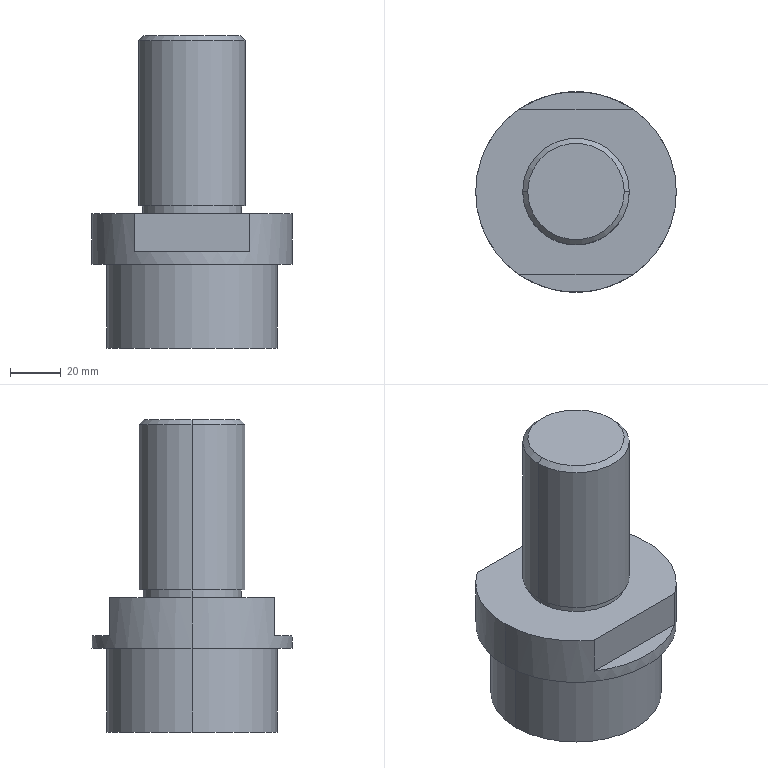Part | SolidWorks | features ICE 4, Chamfer 1, Extrusion 1 | 1 solid | 19 faces | box 79 x 79 x 123 mm | volume 304126 mm3 | plane 9 | cylinder 8 | cone 2 | commonest cylinder face diameters 39 x2 42 x2 67 x2 79 x2
STEP:
#1=CARTESIAN_POINT('',(19.,0.,123.));
#2=VERTEX_POINT('',#1);
#3=CARTESIAN_POINT('',(-19.,0.,123.));
#4=VERTEX_POINT('',#3);
#5=CARTESIAN_POINT('',(0.,0.,123.));
#6=DIRECTION('',(0.,0.,1.));
#7=DIRECTION('',(1.,0.,0.));
#8=AXIS2_PLACEMENT_3D('',#5,#6,#7);
#9=CIRCLE('',#8,19.);
#10=EDGE_CURVE('',#2,#4,#9,.T.);
#11=ORIENTED_EDGE('',*,*,#10,.F.);
#12=CARTESIAN_POINT('',(21.,0.,121.));
#13=VERTEX_POINT('',#12);
#14=CARTESIAN_POINT('',(19.,0.,123.));
#15=DIRECTION('',(0.7071,0.,-0.7071));
#16=VECTOR('',#15,1000.);
#17=LINE('',#14,#16);
#18=EDGE_CURVE('',#2,#13,#17,.T.);
#19=ORIENTED_EDGE('',*,*,#18,.T.);
#20=CARTESIAN_POINT('',(-21.,0.,121.));
#21=VERTEX_POINT('',#20);
#22=CARTESIAN_POINT('',(0.,0.,121.));
#23=DIRECTION('',(0.,0.,-1.));
#24=DIRECTION('',(1.,0.,0.));
#25=AXIS2_PLACEMENT_3D('',#22,#23,#24);
#26=CIRCLE('',#25,21.);
#27=EDGE_CURVE('',#21,#13,#26,.T.);
#28=ORIENTED_EDGE('',*,*,#27,.F.);
#29=CARTESIAN_POINT('',(-19.,0.,123.));
#30=DIRECTION('',(-0.7071,0.,-0.7071));
#31=VECTOR('',#30,1000.);
#32=LINE('',#29,#31);
#33=EDGE_CURVE('',#4,#21,#32,.T.);
#34=ORIENTED_EDGE('',*,*,#33,.F.);
#35=EDGE_LOOP('',(#11,#19,#28,#34));
#36=FACE_OUTER_BOUND('',#35,.T.);
#37=CARTESIAN_POINT('',(0.,0.,123.));
#38=DIRECTION('',(0.,0.,-1.));
#39=DIRECTION('',(-1.,0.,0.));
#40=AXIS2_PLACEMENT_3D('',#37,#38,#39);
#41=CONICAL_SURFACE('',#40,19.,0.7854);
#42=ADVANCED_FACE('',(#36),#41,.T.);
#43=ORIENTED_EDGE('',*,*,#27,.T.);
#44=CARTESIAN_POINT('',(21.,0.,56.));
#45=VERTEX_POINT('',#44);
#46=CARTESIAN_POINT('',(21.,0.,123.));
#47=DIRECTION('',(0.,0.,-1.));
#48=VECTOR('',#47,1000.);
#49=LINE('',#46,#48);
#50=EDGE_CURVE('',#13,#45,#49,.T.);
#51=ORIENTED_EDGE('',*,*,#50,.T.);
#52=CARTESIAN_POINT('',(-21.,0.,56.));
#53=VERTEX_POINT('',#52);
#54=CARTESIAN_POINT('',(0.,0.,56.));
#55=DIRECTION('',(0.,0.,1.));
#56=DIRECTION('',(1.,0.,0.));
#57=AXIS2_PLACEMENT_3D('',#54,#55,#56);
#58=CIRCLE('',#57,21.);
#59=EDGE_CURVE('',#45,#53,#58,.T.);
#60=ORIENTED_EDGE('',*,*,#59,.T.);
#61=CARTESIAN_POINT('',(-21.,0.,123.));
#62=DIRECTION('',(0.,0.,-1.));
#63=VECTOR('',#62,1000.);
#64=LINE('',#61,#63);
#65=EDGE_CURVE('',#21,#53,#64,.T.);
#66=ORIENTED_EDGE('',*,*,#65,.F.);
#67=EDGE_LOOP('',(#43,#51,#60,#66));
#68=FACE_OUTER_BOUND('',#67,.T.);
#69=CARTESIAN_POINT('',(0.,0.,123.));
#70=DIRECTION('',(0.,0.,-1.));
#71=DIRECTION('',(-1.,0.,0.));
#72=AXIS2_PLACEMENT_3D('',#69,#70,#71);
#73=CYLINDRICAL_SURFACE('',#72,21.);
#74=ADVANCED_FACE('',(#68),#73,.T.);
#75=CARTESIAN_POINT('',(19.5,0.,56.));
#76=VERTEX_POINT('',#75);
#77=CARTESIAN_POINT('',(-19.5,0.,56.));
#78=VERTEX_POINT('',#77);
#79=CARTESIAN_POINT('',(0.,0.,56.));
#80=DIRECTION('',(0.,0.,1.));
#81=DIRECTION('',(1.,0.,0.));
#82=AXIS2_PLACEMENT_3D('',#79,#80,#81);
#83=CIRCLE('',#82,19.5);
#84=EDGE_CURVE('',#76,#78,#83,.T.);
#85=ORIENTED_EDGE('',*,*,#84,.F.);
#86=CARTESIAN_POINT('',(19.5,0.,53.));
#87=VERTEX_POINT('',#86);
#88=CARTESIAN_POINT('',(19.5,0.,56.));
#89=DIRECTION('',(0.,0.,-1.));
#90=VECTOR('',#89,1000.);
#91=LINE('',#88,#90);
#92=EDGE_CURVE('',#76,#87,#91,.T.);
#93=ORIENTED_EDGE('',*,*,#92,.T.);
#94=CARTESIAN_POINT('',(-19.5,0.,53.));
#95=VERTEX_POINT('',#94);
#96=CARTESIAN_POINT('',(0.,0.,53.));
#97=DIRECTION('',(0.,0.,1.));
#98=DIRECTION('',(1.,0.,0.));
#99=AXIS2_PLACEMENT_3D('',#96,#97,#98);
#100=CIRCLE('',#99,19.5);
#101=EDGE_CURVE('',#87,#95,#100,.T.);
#102=ORIENTED_EDGE('',*,*,#101,.T.);
#103=CARTESIAN_POINT('',(-19.5,0.,56.));
#104=DIRECTION('',(0.,0.,-1.));
#105=VECTOR('',#104,1000.);
#106=LINE('',#103,#105);
#107=EDGE_CURVE('',#78,#95,#106,.T.);
#108=ORIENTED_EDGE('',*,*,#107,.F.);
#109=EDGE_LOOP('',(#85,#93,#102,#108));
#110=FACE_OUTER_BOUND('',#109,.T.);
#111=CARTESIAN_POINT('',(0.,0.,56.));
#112=DIRECTION('',(0.,0.,-1.));
#113=DIRECTION('',(-1.,0.,0.));
#114=AXIS2_PLACEMENT_3D('',#111,#112,#113);
#115=CYLINDRICAL_SURFACE('',#114,19.5);
#116=ADVANCED_FACE('',(#110),#115,.T.);
#117=CARTESIAN_POINT('',(39.5,0.,53.));
#118=VERTEX_POINT('',#117);
#119=CARTESIAN_POINT('',(22.45,32.5,53.));
#120=VERTEX_POINT('',#119);
#121=CARTESIAN_POINT('',(0.,0.,53.));
#122=DIRECTION('',(0.,0.,1.));
#123=DIRECTION('',(1.,0.,0.));
#124=AXIS2_PLACEMENT_3D('',#121,#122,#123);
#125=CIRCLE('',#124,39.5);
#126=EDGE_CURVE('',#118,#120,#125,.T.);
#127=ORIENTED_EDGE('',*,*,#126,.F.);
#128=CARTESIAN_POINT('',(39.5,0.,33.));
#129=VERTEX_POINT('',#128);
#130=CARTESIAN_POINT('',(39.5,0.,53.));
#131=DIRECTION('',(0.,0.,-1.));
#132=VECTOR('',#131,1000.);
#133=LINE('',#130,#132);
#134=EDGE_CURVE('',#118,#129,#133,.T.);
#135=ORIENTED_EDGE('',*,*,#134,.T.);
#136=CARTESIAN_POINT('',(-39.5,0.,33.));
#137=VERTEX_POINT('',#136);
#138=CARTESIAN_POINT('',(0.,0.,33.));
#139=DIRECTION('',(0.,0.,1.));
#140=DIRECTION('',(1.,0.,0.));
#141=AXIS2_PLACEMENT_3D('',#138,#139,#140);
#142=CIRCLE('',#141,39.5);
#143=EDGE_CURVE('',#129,#137,#142,.T.);
#144=ORIENTED_EDGE('',*,*,#143,.T.);
#145=CARTESIAN_POINT('',(-39.5,0.,53.));
#146=VERTEX_POINT('',#145);
#147=CARTESIAN_POINT('',(-39.5,0.,53.));
#148=DIRECTION('',(0.,0.,-1.));
#149=VECTOR('',#148,1000.);
#150=LINE('',#147,#149);
#151=EDGE_CURVE('',#146,#137,#150,.T.);
#152=ORIENTED_EDGE('',*,*,#151,.F.);
#153=CARTESIAN_POINT('',(-22.45,32.5,53.));
#154=VERTEX_POINT('',#153);
#155=CARTESIAN_POINT('',(0.,0.,53.));
#156=DIRECTION('',(0.,0.,1.));
#157=DIRECTION('',(1.,0.,0.));
#158=AXIS2_PLACEMENT_3D('',#155,#156,#157);
#159=CIRCLE('',#158,39.5);
#160=EDGE_CURVE('',#154,#146,#159,.T.);
#161=ORIENTED_EDGE('',*,*,#160,.F.);
#162=CARTESIAN_POINT('',(-22.45,32.5,38.));
#163=VERTEX_POINT('',#162);
#164=CARTESIAN_POINT('',(-22.45,32.5,38.));
#165=DIRECTION('',(0.,0.,1.));
#166=VECTOR('',#165,1000.);
#167=LINE('',#164,#166);
#168=EDGE_CURVE('',#163,#154,#167,.T.);
#169=ORIENTED_EDGE('',*,*,#168,.F.);
#170=CARTESIAN_POINT('',(22.45,32.5,38.));
#171=VERTEX_POINT('',#170);
#172=CARTESIAN_POINT('',(0.,0.,38.));
#173=DIRECTION('',(0.,0.,1.));
#174=DIRECTION('',(1.,0.,0.));
#175=AXIS2_PLACEMENT_3D('',#172,#173,#174);
#176=CIRCLE('',#175,39.5);
#177=EDGE_CURVE('',#171,#163,#176,.T.);
#178=ORIENTED_EDGE('',*,*,#177,.F.);
#179=CARTESIAN_POINT('',(22.45,32.5,38.));
#180=DIRECTION('',(0.,0.,1.));
#181=VECTOR('',#180,1000.);
#182=LINE('',#179,#181);
#183=EDGE_CURVE('',#171,#120,#182,.T.);
#184=ORIENTED_EDGE('',*,*,#183,.T.);
#185=EDGE_LOOP('',(#127,#135,#144,#152,#161,#169,#178,#184));
#186=FACE_OUTER_BOUND('',#185,.T.);
#187=CARTESIAN_POINT('',(0.,0.,53.));
#188=DIRECTION('',(0.,0.,-1.));
#189=DIRECTION('',(-1.,0.,0.));
#190=AXIS2_PLACEMENT_3D('',#187,#188,#189);
#191=CYLINDRICAL_SURFACE('',#190,39.5);
#192=ADVANCED_FACE('',(#186),#191,.T.);
#193=CARTESIAN_POINT('',(33.5,0.,33.));
#194=VERTEX_POINT('',#193);
#195=CARTESIAN_POINT('',(-33.5,0.,33.));
#196=VERTEX_POINT('',#195);
#197=CARTESIAN_POINT('',(0.,0.,33.));
#198=DIRECTION('',(0.,0.,1.));
#199=DIRECTION('',(1.,0.,0.));
#200=AXIS2_PLACEMENT_3D('',#197,#198,#199);
#201=CIRCLE('',#200,33.5);
#202=EDGE_CURVE('',#194,#196,#201,.T.);
#203=ORIENTED_EDGE('',*,*,#202,.F.);
#204=CARTESIAN_POINT('',(33.5,0.,0.));
#205=VERTEX_POINT('',#204);
#206=CARTESIAN_POINT('',(33.5,0.,33.));
#207=DIRECTION('',(0.,0.,-1.));
#208=VECTOR('',#207,1000.);
#209=LINE('',#206,#208);
#210=EDGE_CURVE('',#194,#205,#209,.T.);
#211=ORIENTED_EDGE('',*,*,#210,.T.);
#212=CARTESIAN_POINT('',(-33.5,0.,0.));
#213=VERTEX_POINT('',#212);
#214=CARTESIAN_POINT('',(0.,0.,0.));
#215=DIRECTION('',(0.,0.,1.));
#216=DIRECTION('',(1.,0.,0.));
#217=AXIS2_PLACEMENT_3D('',#214,#215,#216);
#218=CIRCLE('',#217,33.5);
#219=EDGE_CURVE('',#205,#213,#218,.T.);
#220=ORIENTED_EDGE('',*,*,#219,.T.);
#221=CARTESIAN_POINT('',(-33.5,0.,33.));
#222=DIRECTION('',(0.,0.,-1.));
#223=VECTOR('',#222,1000.);
#224=LINE('',#221,#223);
#225=EDGE_CURVE('',#196,#213,#224,.T.);
#226=ORIENTED_EDGE('',*,*,#225,.F.);
#227=EDGE_LOOP('',(#203,#211,#220,#226));
#228=FACE_OUTER_BOUND('',#227,.T.);
#229=CARTESIAN_POINT('',(0.,0.,33.));
#230=DIRECTION('',(0.,0.,-1.));
#231=DIRECTION('',(-1.,0.,0.));
#232=AXIS2_PLACEMENT_3D('',#229,#230,#231);
#233=CYLINDRICAL_SURFACE('',#232,33.5);
#234=ADVANCED_FACE('',(#228),#233,.T.);
#235=ORIENTED_EDGE('',*,*,#210,.F.);
#236=CARTESIAN_POINT('',(0.,0.,33.));
#237=DIRECTION('',(0.,0.,1.));
#238=DIRECTION('',(1.,0.,0.));
#239=AXIS2_PLACEMENT_3D('',#236,#237,#238);
#240=CIRCLE('',#239,33.5);
#241=EDGE_CURVE('',#196,#194,#240,.T.);
#242=ORIENTED_EDGE('',*,*,#241,.F.);
#243=ORIENTED_EDGE('',*,*,#225,.T.);
#244=CARTESIAN_POINT('',(0.,0.,0.));
#245=DIRECTION('',(0.,0.,1.));
#246=DIRECTION('',(1.,0.,0.));
#247=AXIS2_PLACEMENT_3D('',#244,#245,#246);
#248=CIRCLE('',#247,33.5);
#249=EDGE_CURVE('',#213,#205,#248,.T.);
#250=ORIENTED_EDGE('',*,*,#249,.T.);
#251=EDGE_LOOP('',(#235,#242,#243,#250));
#252=FACE_OUTER_BOUND('',#251,.T.);
#253=CARTESIAN_POINT('',(0.,0.,33.));
#254=DIRECTION('',(0.,0.,-1.));
#255=DIRECTION('',(-1.,0.,0.));
#256=AXIS2_PLACEMENT_3D('',#253,#254,#255);
#257=CYLINDRICAL_SURFACE('',#256,33.5);
#258=ADVANCED_FACE('',(#252),#257,.T.);
#259=ORIENTED_EDGE('',*,*,#249,.F.);
#260=ORIENTED_EDGE('',*,*,#219,.F.);
#261=EDGE_LOOP('',(#259,#260));
#262=FACE_OUTER_BOUND('',#261,.T.);
#263=CARTESIAN_POINT('',(0.,0.,0.));
#264=DIRECTION('',(0.,0.,1.));
#265=DIRECTION('',(1.,0.,0.));
#266=AXIS2_PLACEMENT_3D('',#263,#264,#265);
#267=PLANE('',#266);
#268=ADVANCED_FACE('',(#262),#267,.F.);
#269=ORIENTED_EDGE('',*,*,#134,.F.);
#270=CARTESIAN_POINT('',(22.45,-32.5,53.));
#271=VERTEX_POINT('',#270);
#272=CARTESIAN_POINT('',(0.,0.,53.));
#273=DIRECTION('',(0.,0.,1.));
#274=DIRECTION('',(1.,0.,0.));
#275=AXIS2_PLACEMENT_3D('',#272,#273,#274);
#276=CIRCLE('',#275,39.5);
#277=EDGE_CURVE('',#271,#118,#276,.T.);
#278=ORIENTED_EDGE('',*,*,#277,.F.);
#279=CARTESIAN_POINT('',(22.45,-32.5,38.));
#280=VERTEX_POINT('',#279);
#281=CARTESIAN_POINT('',(22.45,-32.5,38.));
#282=DIRECTION('',(0.,0.,1.));
#283=VECTOR('',#282,1000.);
#284=LINE('',#281,#283);
#285=EDGE_CURVE('',#280,#271,#284,.T.);
#286=ORIENTED_EDGE('',*,*,#285,.F.);
#287=CARTESIAN_POINT('',(-22.45,-32.5,38.));
#288=VERTEX_POINT('',#287);
#289=CARTESIAN_POINT('',(0.,0.,38.));
#290=DIRECTION('',(0.,0.,1.));
#291=DIRECTION('',(1.,0.,0.));
#292=AXIS2_PLACEMENT_3D('',#289,#290,#291);
#293=CIRCLE('',#292,39.5);
#294=EDGE_CURVE('',#288,#280,#293,.T.);
#295=ORIENTED_EDGE('',*,*,#294,.F.);
#296=CARTESIAN_POINT('',(-22.45,-32.5,53.));
#297=VERTEX_POINT('',#296);
#298=CARTESIAN_POINT('',(-22.45,-32.5,38.));
#299=DIRECTION('',(0.,0.,1.));
#300=VECTOR('',#299,1000.);
#301=LINE('',#298,#300);
#302=EDGE_CURVE('',#288,#297,#301,.T.);
#303=ORIENTED_EDGE('',*,*,#302,.T.);
#304=CARTESIAN_POINT('',(0.,0.,53.));
#305=DIRECTION('',(0.,0.,1.));
#306=DIRECTION('',(1.,0.,0.));
#307=AXIS2_PLACEMENT_3D('',#304,#305,#306);
#308=CIRCLE('',#307,39.5);
#309=EDGE_CURVE('',#146,#297,#308,.T.);
#310=ORIENTED_EDGE('',*,*,#309,.F.);
#311=ORIENTED_EDGE('',*,*,#151,.T.);
#312=CARTESIAN_POINT('',(0.,0.,33.));
#313=DIRECTION('',(0.,0.,1.));
#314=DIRECTION('',(1.,0.,0.));
#315=AXIS2_PLACEMENT_3D('',#312,#313,#314);
#316=CIRCLE('',#315,39.5);
#317=EDGE_CURVE('',#137,#129,#316,.T.);
#318=ORIENTED_EDGE('',*,*,#317,.T.);
#319=EDGE_LOOP('',(#269,#278,#286,#295,#303,#310,#311,#318));
#320=FACE_OUTER_BOUND('',#319,.T.);
#321=CARTESIAN_POINT('',(0.,0.,53.));
#322=DIRECTION('',(0.,0.,-1.));
#323=DIRECTION('',(-1.,0.,0.));
#324=AXIS2_PLACEMENT_3D('',#321,#322,#323);
#325=CYLINDRICAL_SURFACE('',#324,39.5);
#326=ADVANCED_FACE('',(#320),#325,.T.);
#327=CARTESIAN_POINT('',(0.,0.,53.));
#328=DIRECTION('',(0.,0.,1.));
#329=DIRECTION('',(1.,0.,0.));
#330=AXIS2_PLACEMENT_3D('',#327,#328,#329);
#331=CIRCLE('',#330,19.5);
#332=EDGE_CURVE('',#95,#87,#331,.T.);
#333=ORIENTED_EDGE('',*,*,#332,.F.);
#334=ORIENTED_EDGE('',*,*,#101,.F.);
#335=EDGE_LOOP('',(#333,#334));
#336=FACE_BOUND('',#335,.T.);
#337=CARTESIAN_POINT('',(-22.45,-32.5,53.));
#338=DIRECTION('',(-1.,0.,0.));
#339=VECTOR('',#338,1000.);
#340=LINE('',#337,#339);
#341=EDGE_CURVE('',#271,#297,#340,.T.);
#342=ORIENTED_EDGE('',*,*,#341,.F.);
#343=ORIENTED_EDGE('',*,*,#277,.T.);
#344=ORIENTED_EDGE('',*,*,#126,.T.);
#345=CARTESIAN_POINT('',(-22.45,32.5,53.));
#346=DIRECTION('',(1.,0.,0.));
#347=VECTOR('',#346,1000.);
#348=LINE('',#345,#347);
#349=EDGE_CURVE('',#154,#120,#348,.T.);
#350=ORIENTED_EDGE('',*,*,#349,.F.);
#351=ORIENTED_EDGE('',*,*,#160,.T.);
#352=ORIENTED_EDGE('',*,*,#309,.T.);
#353=EDGE_LOOP('',(#342,#343,#344,#350,#351,#352));
#354=FACE_OUTER_BOUND('',#353,.T.);
#355=CARTESIAN_POINT('',(0.,0.,53.));
#356=DIRECTION('',(0.,0.,1.));
#357=DIRECTION('',(1.,0.,0.));
#358=AXIS2_PLACEMENT_3D('',#355,#356,#357);
#359=PLANE('',#358);
#360=ADVANCED_FACE('',(#336,#354),#359,.T.);
#361=ORIENTED_EDGE('',*,*,#241,.T.);
#362=ORIENTED_EDGE('',*,*,#202,.T.);
#363=EDGE_LOOP('',(#361,#362));
#364=FACE_BOUND('',#363,.T.);
#365=ORIENTED_EDGE('',*,*,#317,.F.);
#366=ORIENTED_EDGE('',*,*,#143,.F.);
#367=EDGE_LOOP('',(#365,#366));
#368=FACE_OUTER_BOUND('',#367,.T.);
#369=CARTESIAN_POINT('',(0.,0.,33.));
#370=DIRECTION('',(0.,0.,1.));
#371=DIRECTION('',(1.,0.,0.));
#372=AXIS2_PLACEMENT_3D('',#369,#370,#371);
#373=PLANE('',#372);
#374=ADVANCED_FACE('',(#364,#368),#373,.F.);
#375=ORIENTED_EDGE('',*,*,#349,.T.);
#376=ORIENTED_EDGE('',*,*,#183,.F.);
#377=CARTESIAN_POINT('',(-22.45,32.5,38.));
#378=DIRECTION('',(1.,0.,0.));
#379=VECTOR('',#378,1000.);
#380=LINE('',#377,#379);
#381=EDGE_CURVE('',#163,#171,#380,.T.);
#382=ORIENTED_EDGE('',*,*,#381,.F.);
#383=ORIENTED_EDGE('',*,*,#168,.T.);
#384=EDGE_LOOP('',(#375,#376,#382,#383));
#385=FACE_OUTER_BOUND('',#384,.T.);
#386=CARTESIAN_POINT('',(-22.45,32.5,38.));
#387=DIRECTION('',(0.,-1.,0.));
#388=DIRECTION('',(0.,0.,-1.));
#389=AXIS2_PLACEMENT_3D('',#386,#387,#388);
#390=PLANE('',#389);
#391=ADVANCED_FACE('',(#385),#390,.F.);
#392=ORIENTED_EDGE('',*,*,#177,.T.);
#393=ORIENTED_EDGE('',*,*,#381,.T.);
#394=EDGE_LOOP('',(#392,#393));
#395=FACE_OUTER_BOUND('',#394,.T.);
#396=CARTESIAN_POINT('',(0.,0.,38.));
#397=DIRECTION('',(0.,0.,1.));
#398=DIRECTION('',(1.,0.,0.));
#399=AXIS2_PLACEMENT_3D('',#396,#397,#398);
#400=PLANE('',#399);
#401=ADVANCED_FACE('',(#395),#400,.T.);
#402=ORIENTED_EDGE('',*,*,#341,.T.);
#403=ORIENTED_EDGE('',*,*,#302,.F.);
#404=CARTESIAN_POINT('',(-22.45,-32.5,38.));
#405=DIRECTION('',(-1.,0.,0.));
#406=VECTOR('',#405,1000.);
#407=LINE('',#404,#406);
#408=EDGE_CURVE('',#280,#288,#407,.T.);
#409=ORIENTED_EDGE('',*,*,#408,.F.);
#410=ORIENTED_EDGE('',*,*,#285,.T.);
#411=EDGE_LOOP('',(#402,#403,#409,#410));
#412=FACE_OUTER_BOUND('',#411,.T.);
#413=CARTESIAN_POINT('',(-22.45,-32.5,38.));
#414=DIRECTION('',(0.,1.,0.));
#415=DIRECTION('',(0.,0.,1.));
#416=AXIS2_PLACEMENT_3D('',#413,#414,#415);
#417=PLANE('',#416);
#418=ADVANCED_FACE('',(#412),#417,.F.);
#419=ORIENTED_EDGE('',*,*,#294,.T.);
#420=ORIENTED_EDGE('',*,*,#408,.T.);
#421=EDGE_LOOP('',(#419,#420));
#422=FACE_OUTER_BOUND('',#421,.T.);
#423=CARTESIAN_POINT('',(0.,0.,38.));
#424=DIRECTION('',(0.,0.,1.));
#425=DIRECTION('',(1.,0.,0.));
#426=AXIS2_PLACEMENT_3D('',#423,#424,#425);
#427=PLANE('',#426);
#428=ADVANCED_FACE('',(#422),#427,.T.);
#429=ORIENTED_EDGE('',*,*,#92,.F.);
#430=CARTESIAN_POINT('',(0.,0.,56.));
#431=DIRECTION('',(0.,0.,1.));
#432=DIRECTION('',(1.,0.,0.));
#433=AXIS2_PLACEMENT_3D('',#430,#431,#432);
#434=CIRCLE('',#433,19.5);
#435=EDGE_CURVE('',#78,#76,#434,.T.);
#436=ORIENTED_EDGE('',*,*,#435,.F.);
#437=ORIENTED_EDGE('',*,*,#107,.T.);
#438=ORIENTED_EDGE('',*,*,#332,.T.);
#439=EDGE_LOOP('',(#429,#436,#437,#438));
#440=FACE_OUTER_BOUND('',#439,.T.);
#441=CARTESIAN_POINT('',(0.,0.,56.));
#442=DIRECTION('',(0.,0.,-1.));
#443=DIRECTION('',(-1.,0.,0.));
#444=AXIS2_PLACEMENT_3D('',#441,#442,#443);
#445=CYLINDRICAL_SURFACE('',#444,19.5);
#446=ADVANCED_FACE('',(#440),#445,.T.);
#447=ORIENTED_EDGE('',*,*,#50,.F.);
#448=CARTESIAN_POINT('',(0.,0.,121.));
#449=DIRECTION('',(0.,0.,-1.));
#450=DIRECTION('',(1.,0.,0.));
#451=AXIS2_PLACEMENT_3D('',#448,#449,#450);
#452=CIRCLE('',#451,21.);
#453=EDGE_CURVE('',#13,#21,#452,.T.);
#454=ORIENTED_EDGE('',*,*,#453,.T.);
#455=ORIENTED_EDGE('',*,*,#65,.T.);
#456=CARTESIAN_POINT('',(0.,0.,56.));
#457=DIRECTION('',(0.,0.,1.));
#458=DIRECTION('',(1.,0.,0.));
#459=AXIS2_PLACEMENT_3D('',#456,#457,#458);
#460=CIRCLE('',#459,21.);
#461=EDGE_CURVE('',#53,#45,#460,.T.);
#462=ORIENTED_EDGE('',*,*,#461,.T.);
#463=EDGE_LOOP('',(#447,#454,#455,#462));
#464=FACE_OUTER_BOUND('',#463,.T.);
#465=CARTESIAN_POINT('',(0.,0.,123.));
#466=DIRECTION('',(0.,0.,-1.));
#467=DIRECTION('',(-1.,0.,0.));
#468=AXIS2_PLACEMENT_3D('',#465,#466,#467);
#469=CYLINDRICAL_SURFACE('',#468,21.);
#470=ADVANCED_FACE('',(#464),#469,.T.);
#471=CARTESIAN_POINT('',(0.,0.,123.));
#472=DIRECTION('',(0.,0.,1.));
#473=DIRECTION('',(1.,0.,0.));
#474=AXIS2_PLACEMENT_3D('',#471,#472,#473);
#475=CIRCLE('',#474,19.);
#476=EDGE_CURVE('',#4,#2,#475,.T.);
#477=ORIENTED_EDGE('',*,*,#476,.T.);
#478=ORIENTED_EDGE('',*,*,#10,.T.);
#479=EDGE_LOOP('',(#477,#478));
#480=FACE_OUTER_BOUND('',#479,.T.);
#481=CARTESIAN_POINT('',(0.,0.,123.));
#482=DIRECTION('',(0.,0.,1.));
#483=DIRECTION('',(1.,0.,0.));
#484=AXIS2_PLACEMENT_3D('',#481,#482,#483);
#485=PLANE('',#484);
#486=ADVANCED_FACE('',(#480),#485,.T.);
#487=ORIENTED_EDGE('',*,*,#435,.T.);
#488=ORIENTED_EDGE('',*,*,#84,.T.);
#489=EDGE_LOOP('',(#487,#488));
#490=FACE_BOUND('',#489,.T.);
#491=ORIENTED_EDGE('',*,*,#461,.F.);
#492=ORIENTED_EDGE('',*,*,#59,.F.);
#493=EDGE_LOOP('',(#491,#492));
#494=FACE_OUTER_BOUND('',#493,.T.);
#495=CARTESIAN_POINT('',(0.,0.,56.));
#496=DIRECTION('',(0.,0.,1.));
#497=DIRECTION('',(1.,0.,0.));
#498=AXIS2_PLACEMENT_3D('',#495,#496,#497);
#499=PLANE('',#498);
#500=ADVANCED_FACE('',(#490,#494),#499,.F.);
#501=ORIENTED_EDGE('',*,*,#18,.F.);
#502=ORIENTED_EDGE('',*,*,#476,.F.);
#503=ORIENTED_EDGE('',*,*,#33,.T.);
#504=ORIENTED_EDGE('',*,*,#453,.F.);
#505=EDGE_LOOP('',(#501,#502,#503,#504));
#506=FACE_OUTER_BOUND('',#505,.T.);
#507=CARTESIAN_POINT('',(0.,0.,123.));
#508=DIRECTION('',(0.,0.,-1.));
#509=DIRECTION('',(-1.,0.,0.));
#510=AXIS2_PLACEMENT_3D('',#507,#508,#509);
#511=CONICAL_SURFACE('',#510,19.,0.7854);
#512=ADVANCED_FACE('',(#506),#511,.T.);
#513=CLOSED_SHELL('',(#42,#74,#116,#192,#234,#258,#268,#326,#360,#374,#391,#401,#418,#428,#446,#470,#486,#500,#512));
#514=MANIFOLD_SOLID_BREP('',#513);
#515=CARTESIAN_POINT('',(0.,0.,0.));
#516=DIRECTION('',(0.,0.,1.));
#517=DIRECTION('',(1.,0.,0.));
#518=AXIS2_PLACEMENT_3D('',#515,#516,#517);
#519=(LENGTH_UNIT()NAMED_UNIT(*)SI_UNIT(.MILLI.,.METRE.));
#520=UNCERTAINTY_MEASURE_WITH_UNIT(LENGTH_MEASURE(0.00001),#519,'','');
#521=(NAMED_UNIT(*)PLANE_ANGLE_UNIT()SI_UNIT($,.RADIAN.));
#522=(NAMED_UNIT(*)SI_UNIT($,.STERADIAN.)SOLID_ANGLE_UNIT());
#523=(GEOMETRIC_REPRESENTATION_CONTEXT(3)GLOBAL_UNCERTAINTY_ASSIGNED_CONTEXT((#520))GLOBAL_UNIT_ASSIGNED_CONTEXT((#519,#521,#522))REPRESENTATION_CONTEXT('',''));
#524=ADVANCED_BREP_SHAPE_REPRESENTATION('',(#514,#518),#523);